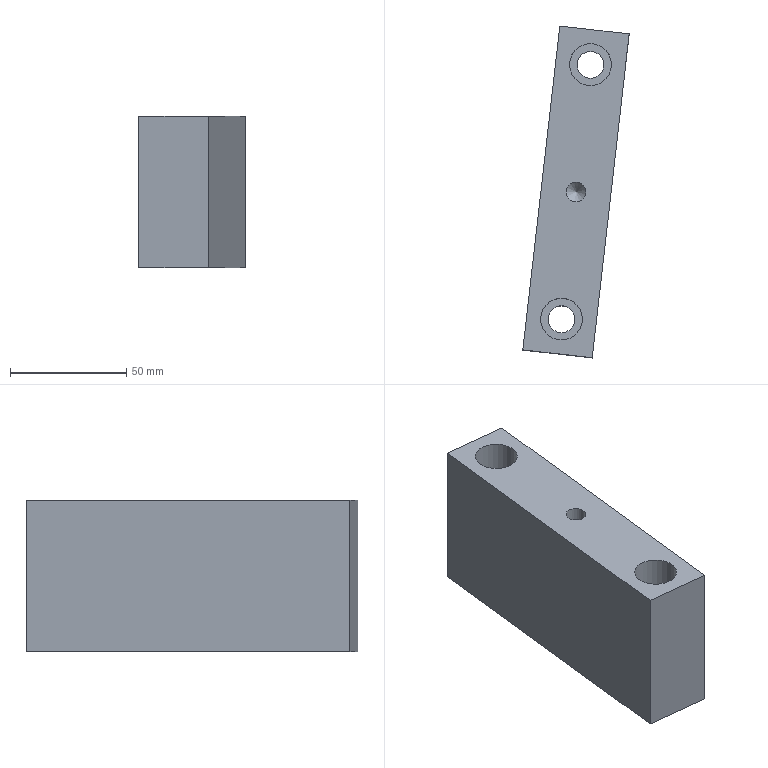Part | NX | features solid 2 | 1 solid | 14 faces | box 45.656 x 142.496 x 65 mm | volume 247863 mm3 | plane 8 | cylinder 5 | cone 1 | commonest cylinder face diameters 11.5 x2 18 x2 8.5 x1
STEP:
#1=CARTESIAN_POINT('',(3114.118,-345.379,-68.));
#2=VERTEX_POINT('',#1);
#3=CARTESIAN_POINT('',(3105.118,-345.379,-68.));
#4=DIRECTION('',(0.,0.,1.));
#5=DIRECTION('',(1.,0.,0.));
#6=AXIS2_PLACEMENT_3D('',#3,#4,#5);
#7=CIRCLE('',#6,9.);
#8=EDGE_CURVE('',#2,#2,#7,.T.);
#9=ORIENTED_EDGE('',*,*,#8,.F.);
#10=EDGE_LOOP('',(#9));
#11=FACE_BOUND('',#10,.T.);
#12=CARTESIAN_POINT('',(3126.571,-236.086,-68.));
#13=VERTEX_POINT('',#12);
#14=CARTESIAN_POINT('',(3117.571,-236.086,-68.));
#15=DIRECTION('',(0.,0.,-1.));
#16=DIRECTION('',(1.,0.,0.));
#17=AXIS2_PLACEMENT_3D('',#14,#15,#16);
#18=CIRCLE('',#17,9.);
#19=EDGE_CURVE('',#13,#13,#18,.T.);
#20=ORIENTED_EDGE('',*,*,#19,.T.);
#21=EDGE_LOOP('',(#20));
#22=FACE_BOUND('',#21,.T.);
#23=CARTESIAN_POINT('',(3134.172,-222.881,-68.));
#24=VERTEX_POINT('',#23);
#25=CARTESIAN_POINT('',(3104.365,-219.484,-68.));
#26=VERTEX_POINT('',#25);
#27=CARTESIAN_POINT('',(3134.172,-222.881,-68.));
#28=DIRECTION('',(-0.9936,0.1132,0.));
#29=VECTOR('',#28,1000.);
#30=LINE('',#27,#29);
#31=EDGE_CURVE('',#24,#26,#30,.T.);
#32=ORIENTED_EDGE('',*,*,#31,.T.);
#33=CARTESIAN_POINT('',(3088.517,-358.585,-68.));
#34=VERTEX_POINT('',#33);
#35=CARTESIAN_POINT('',(2953.003,-1547.968,-68.));
#36=DIRECTION('',(-0.1132,-0.9936,0.));
#37=VECTOR('',#36,1000.);
#38=LINE('',#35,#37);
#39=EDGE_CURVE('',#26,#34,#38,.T.);
#40=ORIENTED_EDGE('',*,*,#39,.T.);
#41=CARTESIAN_POINT('',(3118.324,-361.981,-68.));
#42=VERTEX_POINT('',#41);
#43=CARTESIAN_POINT('',(3118.324,-361.981,-68.));
#44=DIRECTION('',(0.9936,-0.1132,0.));
#45=VECTOR('',#44,1000.);
#46=LINE('',#43,#45);
#47=EDGE_CURVE('',#34,#42,#46,.T.);
#48=ORIENTED_EDGE('',*,*,#47,.T.);
#49=CARTESIAN_POINT('',(3125.682,-297.398,-68.));
#50=DIRECTION('',(-0.1132,-0.9936,0.));
#51=VECTOR('',#50,1000.);
#52=LINE('',#49,#51);
#53=EDGE_CURVE('',#24,#42,#52,.T.);
#54=ORIENTED_EDGE('',*,*,#53,.F.);
#55=EDGE_LOOP('',(#32,#40,#48,#54));
#56=FACE_BOUND('',#55,.T.);
#57=CARTESIAN_POINT('',(3115.594,-290.733,-68.));
#58=VERTEX_POINT('',#57);
#59=CARTESIAN_POINT('',(3111.344,-290.733,-68.));
#60=DIRECTION('',(0.,0.,1.));
#61=DIRECTION('',(1.,0.,0.));
#62=AXIS2_PLACEMENT_3D('',#59,#60,#61);
#63=CIRCLE('',#62,4.25);
#64=EDGE_CURVE('',#58,#58,#63,.T.);
#65=ORIENTED_EDGE('',*,*,#64,.F.);
#66=EDGE_LOOP('',(#65));
#67=FACE_BOUND('',#66,.T.);
#68=CARTESIAN_POINT('',(3125.682,-297.398,-68.));
#69=DIRECTION('',(0.,0.,1.));
#70=DIRECTION('',(-1.,0.,0.));
#71=AXIS2_PLACEMENT_3D('',#68,#69,#70);
#72=PLANE('',#71);
#73=ADVANCED_FACE('',(#11,#22,#56,#67),#72,.T.);
#74=CARTESIAN_POINT('',(3118.324,-361.981,-133.));
#75=VERTEX_POINT('',#74);
#76=CARTESIAN_POINT('',(3088.517,-358.585,-133.));
#77=VERTEX_POINT('',#76);
#78=CARTESIAN_POINT('',(3118.324,-361.981,-133.));
#79=DIRECTION('',(-0.9936,0.1132,0.));
#80=VECTOR('',#79,1000.);
#81=LINE('',#78,#80);
#82=EDGE_CURVE('',#75,#77,#81,.T.);
#83=ORIENTED_EDGE('',*,*,#82,.T.);
#84=CARTESIAN_POINT('',(3104.365,-219.484,-133.));
#85=VERTEX_POINT('',#84);
#86=CARTESIAN_POINT('',(2953.003,-1547.968,-133.));
#87=DIRECTION('',(0.1132,0.9936,0.));
#88=VECTOR('',#87,1000.);
#89=LINE('',#86,#88);
#90=EDGE_CURVE('',#77,#85,#89,.T.);
#91=ORIENTED_EDGE('',*,*,#90,.T.);
#92=CARTESIAN_POINT('',(3134.172,-222.881,-133.));
#93=VERTEX_POINT('',#92);
#94=CARTESIAN_POINT('',(3134.172,-222.881,-133.));
#95=DIRECTION('',(0.9936,-0.1132,0.));
#96=VECTOR('',#95,1000.);
#97=LINE('',#94,#96);
#98=EDGE_CURVE('',#85,#93,#97,.T.);
#99=ORIENTED_EDGE('',*,*,#98,.T.);
#100=CARTESIAN_POINT('',(3154.041,-48.491,-133.));
#101=DIRECTION('',(0.1132,0.9936,0.));
#102=VECTOR('',#101,1000.);
#103=LINE('',#100,#102);
#104=EDGE_CURVE('',#75,#93,#103,.T.);
#105=ORIENTED_EDGE('',*,*,#104,.F.);
#106=EDGE_LOOP('',(#83,#91,#99,#105));
#107=FACE_BOUND('',#106,.T.);
#108=CARTESIAN_POINT('',(3111.821,-236.086,-133.));
#109=VERTEX_POINT('',#108);
#110=CARTESIAN_POINT('',(3117.571,-236.086,-133.));
#111=DIRECTION('',(0.,0.,1.));
#112=DIRECTION('',(-1.,0.,0.));
#113=AXIS2_PLACEMENT_3D('',#110,#111,#112);
#114=CIRCLE('',#113,5.75);
#115=EDGE_CURVE('',#109,#109,#114,.T.);
#116=ORIENTED_EDGE('',*,*,#115,.T.);
#117=EDGE_LOOP('',(#116));
#118=FACE_BOUND('',#117,.T.);
#119=CARTESIAN_POINT('',(3099.368,-345.379,-133.));
#120=VERTEX_POINT('',#119);
#121=CARTESIAN_POINT('',(3105.118,-345.379,-133.));
#122=DIRECTION('',(0.,0.,-1.));
#123=DIRECTION('',(-1.,0.,0.));
#124=AXIS2_PLACEMENT_3D('',#121,#122,#123);
#125=CIRCLE('',#124,5.75);
#126=EDGE_CURVE('',#120,#120,#125,.T.);
#127=ORIENTED_EDGE('',*,*,#126,.F.);
#128=EDGE_LOOP('',(#127));
#129=FACE_BOUND('',#128,.T.);
#130=CARTESIAN_POINT('',(1034.5,193.,-133.));
#131=DIRECTION('',(0.,0.,-1.));
#132=DIRECTION('',(-1.,0.,0.));
#133=AXIS2_PLACEMENT_3D('',#130,#131,#132);
#134=PLANE('',#133);
#135=ADVANCED_FACE('',(#107,#118,#129),#134,.T.);
#136=ORIENTED_EDGE('',*,*,#104,.T.);
#137=CARTESIAN_POINT('',(3134.172,-222.881,-123.));
#138=DIRECTION('',(-0.000000001,0.,1.));
#139=VECTOR('',#138,1000.);
#140=LINE('',#137,#139);
#141=EDGE_CURVE('',#93,#24,#140,.T.);
#142=ORIENTED_EDGE('',*,*,#141,.T.);
#143=ORIENTED_EDGE('',*,*,#53,.T.);
#144=CARTESIAN_POINT('',(3118.324,-361.981,-123.));
#145=DIRECTION('',(0.000000001,0.,-1.));
#146=VECTOR('',#145,1000.);
#147=LINE('',#144,#146);
#148=EDGE_CURVE('',#42,#75,#147,.T.);
#149=ORIENTED_EDGE('',*,*,#148,.T.);
#150=EDGE_LOOP('',(#136,#142,#143,#149));
#151=FACE_BOUND('',#150,.T.);
#152=CARTESIAN_POINT('',(3128.069,-276.448,-65.201));
#153=DIRECTION('',(0.9936,-0.1132,0.000000001));
#154=DIRECTION('',(0.1132,0.9936,0.));
#155=AXIS2_PLACEMENT_3D('',#152,#153,#154);
#156=PLANE('',#155);
#157=ADVANCED_FACE('',(#151),#156,.T.);
#158=ORIENTED_EDGE('',*,*,#47,.F.);
#159=CARTESIAN_POINT('',(3088.517,-358.585,-123.));
#160=DIRECTION('',(-0.000000001,0.,1.));
#161=VECTOR('',#160,1000.);
#162=LINE('',#159,#161);
#163=EDGE_CURVE('',#77,#34,#162,.T.);
#164=ORIENTED_EDGE('',*,*,#163,.F.);
#165=ORIENTED_EDGE('',*,*,#82,.F.);
#166=ORIENTED_EDGE('',*,*,#148,.F.);
#167=EDGE_LOOP('',(#158,#164,#165,#166));
#168=FACE_BOUND('',#167,.T.);
#169=CARTESIAN_POINT('',(3118.324,-361.981,-123.));
#170=DIRECTION('',(-0.1132,-0.9936,0.));
#171=DIRECTION('',(0.9936,-0.1132,0.));
#172=AXIS2_PLACEMENT_3D('',#169,#170,#171);
#173=PLANE('',#172);
#174=ADVANCED_FACE('',(#168),#173,.T.);
#175=ORIENTED_EDGE('',*,*,#98,.F.);
#176=CARTESIAN_POINT('',(3104.365,-219.484,-706.6));
#177=DIRECTION('',(-0.000000001,0.,1.));
#178=VECTOR('',#177,1000.);
#179=LINE('',#176,#178);
#180=EDGE_CURVE('',#85,#26,#179,.T.);
#181=ORIENTED_EDGE('',*,*,#180,.T.);
#182=ORIENTED_EDGE('',*,*,#31,.F.);
#183=ORIENTED_EDGE('',*,*,#141,.F.);
#184=EDGE_LOOP('',(#175,#181,#182,#183));
#185=FACE_BOUND('',#184,.T.);
#186=CARTESIAN_POINT('',(3134.172,-222.881,-123.));
#187=DIRECTION('',(0.1132,0.9936,0.));
#188=DIRECTION('',(-0.9936,0.1132,0.));
#189=AXIS2_PLACEMENT_3D('',#186,#187,#188);
#190=PLANE('',#189);
#191=ADVANCED_FACE('',(#185),#190,.T.);
#192=ORIENTED_EDGE('',*,*,#163,.T.);
#193=ORIENTED_EDGE('',*,*,#39,.F.);
#194=ORIENTED_EDGE('',*,*,#180,.F.);
#195=ORIENTED_EDGE('',*,*,#90,.F.);
#196=EDGE_LOOP('',(#192,#193,#194,#195));
#197=FACE_BOUND('',#196,.T.);
#198=CARTESIAN_POINT('',(2953.003,-1547.968,-706.6));
#199=DIRECTION('',(0.9936,-0.1132,0.000000001));
#200=DIRECTION('',(0.000000001,0.000000001,-1.));
#201=AXIS2_PLACEMENT_3D('',#198,#199,#200);
#202=PLANE('',#201);
#203=ADVANCED_FACE('',(#197),#202,.F.);
#204=CARTESIAN_POINT('',(3111.821,-236.086,-103.));
#205=VERTEX_POINT('',#204);
#206=CARTESIAN_POINT('',(3117.571,-236.086,-103.));
#207=DIRECTION('',(0.,0.,-1.));
#208=DIRECTION('',(-1.,0.,0.));
#209=AXIS2_PLACEMENT_3D('',#206,#207,#208);
#210=CIRCLE('',#209,5.75);
#211=EDGE_CURVE('',#205,#205,#210,.T.);
#212=ORIENTED_EDGE('',*,*,#211,.F.);
#213=EDGE_LOOP('',(#212));
#214=FACE_BOUND('',#213,.T.);
#215=ORIENTED_EDGE('',*,*,#115,.F.);
#216=EDGE_LOOP('',(#215));
#217=FACE_BOUND('',#216,.T.);
#218=CARTESIAN_POINT('',(3117.571,-236.086,-73.));
#219=DIRECTION('',(0.,0.,-1.));
#220=DIRECTION('',(-0.9744,0.225,0.));
#221=AXIS2_PLACEMENT_3D('',#218,#219,#220);
#222=CYLINDRICAL_SURFACE('',#221,5.75);
#223=ADVANCED_FACE('',(#214,#217),#222,.F.);
#224=ORIENTED_EDGE('',*,*,#211,.T.);
#225=EDGE_LOOP('',(#224));
#226=FACE_BOUND('',#225,.T.);
#227=CARTESIAN_POINT('',(3108.571,-236.086,-103.));
#228=VERTEX_POINT('',#227);
#229=CARTESIAN_POINT('',(3117.571,-236.086,-103.));
#230=DIRECTION('',(0.,0.,-1.));
#231=DIRECTION('',(-1.,0.,0.));
#232=AXIS2_PLACEMENT_3D('',#229,#230,#231);
#233=CIRCLE('',#232,9.);
#234=EDGE_CURVE('',#228,#228,#233,.T.);
#235=ORIENTED_EDGE('',*,*,#234,.F.);
#236=EDGE_LOOP('',(#235));
#237=FACE_BOUND('',#236,.T.);
#238=CARTESIAN_POINT('',(3116.681,-235.985,-103.));
#239=DIRECTION('',(0.,0.,-1.));
#240=DIRECTION('',(0.9744,-0.225,0.));
#241=AXIS2_PLACEMENT_3D('',#238,#239,#240);
#242=PLANE('',#241);
#243=ADVANCED_FACE('',(#226,#237),#242,.F.);
#244=ORIENTED_EDGE('',*,*,#234,.T.);
#245=EDGE_LOOP('',(#244));
#246=FACE_BOUND('',#245,.T.);
#247=ORIENTED_EDGE('',*,*,#19,.F.);
#248=EDGE_LOOP('',(#247));
#249=FACE_BOUND('',#248,.T.);
#250=CARTESIAN_POINT('',(3117.571,-236.086,-73.));
#251=DIRECTION('',(0.,0.,-1.));
#252=DIRECTION('',(-0.9744,0.225,0.));
#253=AXIS2_PLACEMENT_3D('',#250,#251,#252);
#254=CYLINDRICAL_SURFACE('',#253,9.);
#255=ADVANCED_FACE('',(#246,#249),#254,.F.);
#256=CARTESIAN_POINT('',(3099.368,-345.379,-103.));
#257=VERTEX_POINT('',#256);
#258=CARTESIAN_POINT('',(3105.118,-345.379,-103.));
#259=DIRECTION('',(0.,0.,1.));
#260=DIRECTION('',(-1.,0.,0.));
#261=AXIS2_PLACEMENT_3D('',#258,#259,#260);
#262=CIRCLE('',#261,5.75);
#263=EDGE_CURVE('',#257,#257,#262,.T.);
#264=ORIENTED_EDGE('',*,*,#263,.T.);
#265=EDGE_LOOP('',(#264));
#266=FACE_BOUND('',#265,.T.);
#267=ORIENTED_EDGE('',*,*,#126,.T.);
#268=EDGE_LOOP('',(#267));
#269=FACE_BOUND('',#268,.T.);
#270=CARTESIAN_POINT('',(3105.118,-345.379,-73.));
#271=DIRECTION('',(0.,0.,-1.));
#272=DIRECTION('',(-1.,0.,0.));
#273=AXIS2_PLACEMENT_3D('',#270,#271,#272);
#274=CYLINDRICAL_SURFACE('',#273,5.75);
#275=ADVANCED_FACE('',(#266,#269),#274,.F.);
#276=ORIENTED_EDGE('',*,*,#263,.F.);
#277=EDGE_LOOP('',(#276));
#278=FACE_BOUND('',#277,.T.);
#279=CARTESIAN_POINT('',(3096.118,-345.379,-103.));
#280=VERTEX_POINT('',#279);
#281=CARTESIAN_POINT('',(3105.118,-345.379,-103.));
#282=DIRECTION('',(0.,0.,1.));
#283=DIRECTION('',(-1.,0.,0.));
#284=AXIS2_PLACEMENT_3D('',#281,#282,#283);
#285=CIRCLE('',#284,9.);
#286=EDGE_CURVE('',#280,#280,#285,.T.);
#287=ORIENTED_EDGE('',*,*,#286,.T.);
#288=EDGE_LOOP('',(#287));
#289=FACE_BOUND('',#288,.T.);
#290=CARTESIAN_POINT('',(3104.228,-345.278,-103.));
#291=DIRECTION('',(0.,0.,-1.));
#292=DIRECTION('',(1.,0.,0.));
#293=AXIS2_PLACEMENT_3D('',#290,#291,#292);
#294=PLANE('',#293);
#295=ADVANCED_FACE('',(#278,#289),#294,.F.);
#296=ORIENTED_EDGE('',*,*,#286,.F.);
#297=EDGE_LOOP('',(#296));
#298=FACE_BOUND('',#297,.T.);
#299=ORIENTED_EDGE('',*,*,#8,.T.);
#300=EDGE_LOOP('',(#299));
#301=FACE_BOUND('',#300,.T.);
#302=CARTESIAN_POINT('',(3105.118,-345.379,-73.));
#303=DIRECTION('',(0.,0.,-1.));
#304=DIRECTION('',(-1.,0.,0.));
#305=AXIS2_PLACEMENT_3D('',#302,#303,#304);
#306=CYLINDRICAL_SURFACE('',#305,9.);
#307=ADVANCED_FACE('',(#298,#301),#306,.F.);
#308=CARTESIAN_POINT('',(3115.594,-290.733,-85.821));
#309=VERTEX_POINT('',#308);
#310=CARTESIAN_POINT('',(3111.344,-290.733,-85.821));
#311=DIRECTION('',(0.,0.,1.));
#312=DIRECTION('',(1.,0.,0.));
#313=AXIS2_PLACEMENT_3D('',#310,#311,#312);
#314=CIRCLE('',#313,4.25);
#315=EDGE_CURVE('',#309,#309,#314,.T.);
#316=ORIENTED_EDGE('',*,*,#315,.F.);
#317=EDGE_LOOP('',(#316));
#318=FACE_BOUND('',#317,.T.);
#319=ORIENTED_EDGE('',*,*,#64,.T.);
#320=EDGE_LOOP('',(#319));
#321=FACE_BOUND('',#320,.T.);
#322=CARTESIAN_POINT('',(3111.344,-290.733,-68.));
#323=DIRECTION('',(0.,0.,-1.));
#324=DIRECTION('',(-1.,0.,0.));
#325=AXIS2_PLACEMENT_3D('',#322,#323,#324);
#326=CYLINDRICAL_SURFACE('',#325,4.25);
#327=ADVANCED_FACE('',(#318,#321),#326,.F.);
#328=CARTESIAN_POINT('',(3111.344,-290.733,-90.071));
#329=VERTEX_POINT('',#328);
#330=VERTEX_LOOP('',#329);
#331=FACE_BOUND('',#330,.T.);
#332=ORIENTED_EDGE('',*,*,#315,.T.);
#333=EDGE_LOOP('',(#332));
#334=FACE_BOUND('',#333,.T.);
#335=CARTESIAN_POINT('',(3111.344,-290.733,-82.286));
#336=DIRECTION('',(0.,0.,1.));
#337=DIRECTION('',(-1.,0.,0.));
#338=AXIS2_PLACEMENT_3D('',#335,#336,#337);
#339=CONICAL_SURFACE('',#338,7.786,0.7854);
#340=ADVANCED_FACE('',(#331,#334),#339,.F.);
#341=CLOSED_SHELL('',(#73,#135,#157,#174,#191,#203,#223,#243,#255,#275,#295,#307,#327,#340));
#342=MANIFOLD_SOLID_BREP('',#341);
#343=(LENGTH_UNIT()NAMED_UNIT(*)SI_UNIT(.MILLI.,.METRE.));
#344=UNCERTAINTY_MEASURE_WITH_UNIT(LENGTH_MEASURE(0.00001),#343,'','');
#345=(NAMED_UNIT(*)PLANE_ANGLE_UNIT()SI_UNIT($,.RADIAN.));
#346=(NAMED_UNIT(*)SI_UNIT($,.STERADIAN.)SOLID_ANGLE_UNIT());
#347=(GEOMETRIC_REPRESENTATION_CONTEXT(3)GLOBAL_UNCERTAINTY_ASSIGNED_CONTEXT((#344))GLOBAL_UNIT_ASSIGNED_CONTEXT((#343,#345,#346))REPRESENTATION_CONTEXT('',''));
#348=ADVANCED_BREP_SHAPE_REPRESENTATION('',(#342),#347);